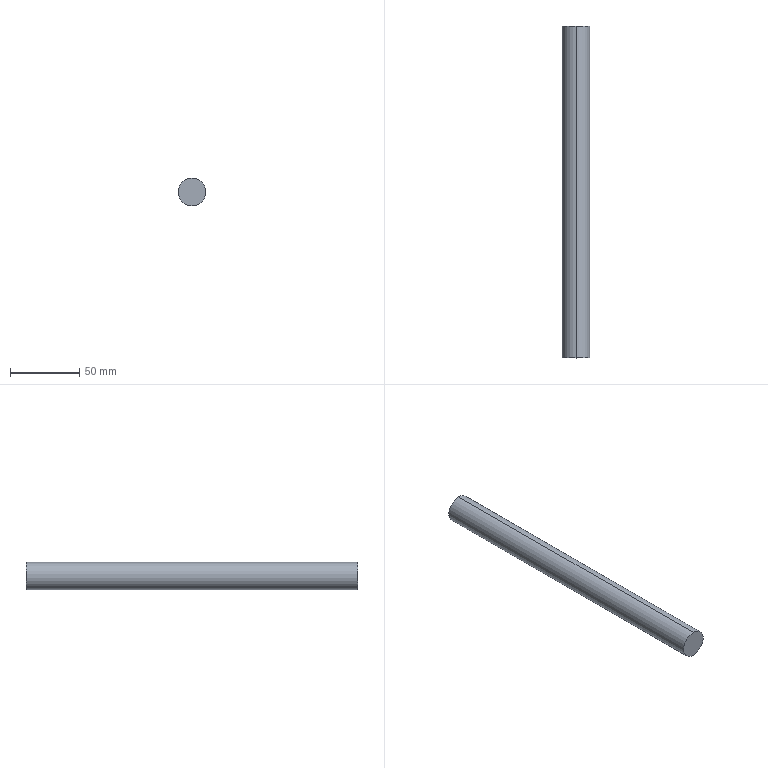Part | STEP file | SYL_0392D6J1SYL0380DJ1006-79820 | 1 solid | 4 faces | box 20 x 240 x 20 mm | volume 75398 mm3 | plane 2 | cylinder 2 | commonest cylinder face diameters 20 x2
STEP:
#1=CARTESIAN_POINT('',(0.,120.,10.));
#2=VERTEX_POINT('',#1);
#3=CARTESIAN_POINT('',(0.,120.,-10.));
#4=VERTEX_POINT('',#3);
#5=CARTESIAN_POINT('',(0.,120.,0.));
#6=DIRECTION('',(0.,1.,0.));
#7=DIRECTION('',(0.,0.,1.));
#8=AXIS2_PLACEMENT_3D('',#5,#6,#7);
#9=CIRCLE('',#8,10.);
#10=EDGE_CURVE('',#2,#4,#9,.T.);
#11=ORIENTED_EDGE('',*,*,#10,.T.);
#12=CARTESIAN_POINT('',(0.,120.,0.));
#13=DIRECTION('',(0.,1.,0.));
#14=DIRECTION('',(0.,0.,-1.));
#15=AXIS2_PLACEMENT_3D('',#12,#13,#14);
#16=CIRCLE('',#15,10.);
#17=EDGE_CURVE('',#4,#2,#16,.T.);
#18=ORIENTED_EDGE('',*,*,#17,.T.);
#19=EDGE_LOOP('',(#11,#18));
#20=FACE_OUTER_BOUND('',#19,.T.);
#21=CARTESIAN_POINT('',(0.,120.,0.));
#22=DIRECTION('',(0.,1.,0.));
#23=DIRECTION('',(1.,0.,0.));
#24=AXIS2_PLACEMENT_3D('',#21,#22,#23);
#25=PLANE('',#24);
#26=ADVANCED_FACE('',(#20),#25,.T.);
#27=CARTESIAN_POINT('',(0.,-120.,10.));
#28=VERTEX_POINT('',#27);
#29=CARTESIAN_POINT('',(0.,-120.,-10.));
#30=VERTEX_POINT('',#29);
#31=CARTESIAN_POINT('',(0.,-120.,0.));
#32=DIRECTION('',(0.,-1.,0.));
#33=DIRECTION('',(0.,0.,1.));
#34=AXIS2_PLACEMENT_3D('',#31,#32,#33);
#35=CIRCLE('',#34,10.);
#36=EDGE_CURVE('',#28,#30,#35,.T.);
#37=ORIENTED_EDGE('',*,*,#36,.F.);
#38=CARTESIAN_POINT('',(0.,120.,10.));
#39=DIRECTION('',(0.,-1.,0.));
#40=VECTOR('',#39,1000.);
#41=LINE('',#38,#40);
#42=EDGE_CURVE('',#2,#28,#41,.T.);
#43=ORIENTED_EDGE('',*,*,#42,.F.);
#44=ORIENTED_EDGE('',*,*,#17,.F.);
#45=CARTESIAN_POINT('',(0.,120.,-10.));
#46=DIRECTION('',(0.,-1.,0.));
#47=VECTOR('',#46,1000.);
#48=LINE('',#45,#47);
#49=EDGE_CURVE('',#4,#30,#48,.T.);
#50=ORIENTED_EDGE('',*,*,#49,.T.);
#51=EDGE_LOOP('',(#37,#43,#44,#50));
#52=FACE_OUTER_BOUND('',#51,.T.);
#53=CARTESIAN_POINT('',(0.,-120.,0.));
#54=DIRECTION('',(0.,1.,0.));
#55=DIRECTION('',(0.,0.,1.));
#56=AXIS2_PLACEMENT_3D('',#53,#54,#55);
#57=CYLINDRICAL_SURFACE('',#56,10.);
#58=ADVANCED_FACE('',(#52),#57,.T.);
#59=ORIENTED_EDGE('',*,*,#49,.F.);
#60=ORIENTED_EDGE('',*,*,#10,.F.);
#61=ORIENTED_EDGE('',*,*,#42,.T.);
#62=CARTESIAN_POINT('',(0.,-120.,0.));
#63=DIRECTION('',(0.,-1.,0.));
#64=DIRECTION('',(0.,0.,-1.));
#65=AXIS2_PLACEMENT_3D('',#62,#63,#64);
#66=CIRCLE('',#65,10.);
#67=EDGE_CURVE('',#30,#28,#66,.T.);
#68=ORIENTED_EDGE('',*,*,#67,.F.);
#69=EDGE_LOOP('',(#59,#60,#61,#68));
#70=FACE_OUTER_BOUND('',#69,.T.);
#71=CARTESIAN_POINT('',(0.,-120.,0.));
#72=DIRECTION('',(0.,1.,0.));
#73=DIRECTION('',(0.,0.,1.));
#74=AXIS2_PLACEMENT_3D('',#71,#72,#73);
#75=CYLINDRICAL_SURFACE('',#74,10.);
#76=ADVANCED_FACE('',(#70),#75,.T.);
#77=ORIENTED_EDGE('',*,*,#36,.T.);
#78=ORIENTED_EDGE('',*,*,#67,.T.);
#79=EDGE_LOOP('',(#77,#78));
#80=FACE_OUTER_BOUND('',#79,.T.);
#81=CARTESIAN_POINT('',(0.,-120.,0.));
#82=DIRECTION('',(0.,1.,0.));
#83=DIRECTION('',(1.,0.,0.));
#84=AXIS2_PLACEMENT_3D('',#81,#82,#83);
#85=PLANE('',#84);
#86=ADVANCED_FACE('',(#80),#85,.F.);
#87=CLOSED_SHELL('',(#26,#58,#76,#86));
#88=MANIFOLD_SOLID_BREP('',#87);
#89=CARTESIAN_POINT('',(0.,0.,0.));
#90=DIRECTION('',(0.,0.,1.));
#91=DIRECTION('',(1.,0.,0.));
#92=AXIS2_PLACEMENT_3D('',#89,#90,#91);
#93=(LENGTH_UNIT()NAMED_UNIT(*)SI_UNIT(.MILLI.,.METRE.));
#94=UNCERTAINTY_MEASURE_WITH_UNIT(LENGTH_MEASURE(0.00001),#93,'','');
#95=(NAMED_UNIT(*)PLANE_ANGLE_UNIT()SI_UNIT($,.RADIAN.));
#96=(NAMED_UNIT(*)SI_UNIT($,.STERADIAN.)SOLID_ANGLE_UNIT());
#97=(GEOMETRIC_REPRESENTATION_CONTEXT(3)GLOBAL_UNCERTAINTY_ASSIGNED_CONTEXT((#94))GLOBAL_UNIT_ASSIGNED_CONTEXT((#93,#95,#96))REPRESENTATION_CONTEXT('',''));
#98=ADVANCED_BREP_SHAPE_REPRESENTATION('',(#88,#92),#97);